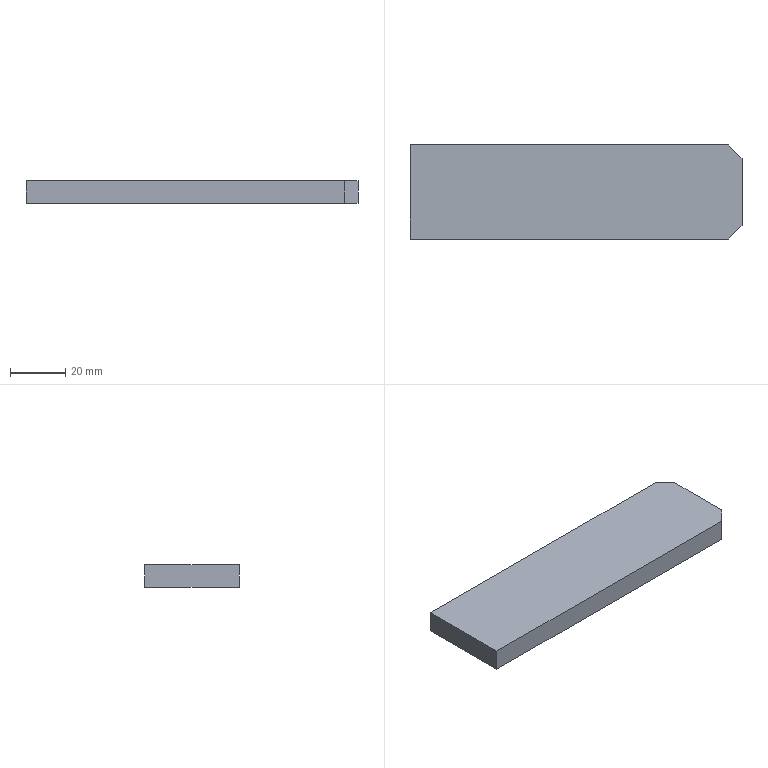Part | STEP file | ASND-0110-Body 1-1-1 | 1 solid | 8 faces | box 120 x 34 x 8 mm | volume 32440 mm3 | plane 8
STEP:
#1=CARTESIAN_POINT('',(0.,0.,0.));
#2=DIRECTION('',(0.,0.,1.));
#3=DIRECTION('',(1.,0.,0.));
#4=AXIS2_PLACEMENT_3D('',#1,#2,#3);
#5=CARTESIAN_POINT('',(115.,34.,8.));
#6=VERTEX_POINT('',#5);
#7=CARTESIAN_POINT('',(120.,29.,8.));
#8=VERTEX_POINT('',#7);
#9=CARTESIAN_POINT('',(115.,34.,8.));
#10=DIRECTION('',(0.7071,-0.7071,0.));
#11=VECTOR('',#10,1.);
#12=LINE('',#9,#11);
#13=CARTESIAN_POINT('',(117.5,31.5,0.));
#14=DIRECTION('',(0.7071,0.7071,0.));
#15=DIRECTION('',(-0.5774,0.5774,0.5774));
#16=AXIS2_PLACEMENT_3D('',#13,#14,#15);
#17=PLANE('',#16);
#18=CARTESIAN_POINT('',(7.506,4.491));
#19=DIRECTION('',(-0.8165,0.5774));
#20=VECTOR('',#19,1.);
#21=LINE('',#18,#20);
#22=(GEOMETRIC_REPRESENTATION_CONTEXT(2)PARAMETRIC_REPRESENTATION_CONTEXT()REPRESENTATION_CONTEXT('',''));
#23=DEFINITIONAL_REPRESENTATION('',(#21),#22);
#24=PCURVE('',#17,#23);
#25=CARTESIAN_POINT('',(50.,25.,8.));
#26=DIRECTION('',(0.,0.,1.));
#27=DIRECTION('',(0.7071,0.7071,0.));
#28=AXIS2_PLACEMENT_3D('',#25,#26,#27);
#29=PLANE('',#28);
#30=CARTESIAN_POINT('',(52.326,-39.598));
#31=DIRECTION('',(0.,-1.));
#32=VECTOR('',#31,1.);
#33=LINE('',#30,#32);
#34=(GEOMETRIC_REPRESENTATION_CONTEXT(2)PARAMETRIC_REPRESENTATION_CONTEXT()REPRESENTATION_CONTEXT('',''));
#35=DEFINITIONAL_REPRESENTATION('',(#33),#34);
#36=PCURVE('',#29,#35);
#37=SURFACE_CURVE('',#12,(#24,#36),.PCURVE_S1.);
#38=EDGE_CURVE('',#6,#8,#37,.T.);
#39=ORIENTED_EDGE('',*,*,#38,.T.);
#40=CARTESIAN_POINT('',(120.,29.,0.));
#41=VERTEX_POINT('',#40);
#42=CARTESIAN_POINT('',(120.,29.,8.));
#43=DIRECTION('',(0.,0.,-1.));
#44=VECTOR('',#43,1.);
#45=LINE('',#42,#44);
#46=CARTESIAN_POINT('',(1.732,8.573));
#47=DIRECTION('',(-0.5774,-0.8165));
#48=VECTOR('',#47,1.);
#49=LINE('',#46,#48);
#50=(GEOMETRIC_REPRESENTATION_CONTEXT(2)PARAMETRIC_REPRESENTATION_CONTEXT()REPRESENTATION_CONTEXT('',''));
#51=DEFINITIONAL_REPRESENTATION('',(#49),#50);
#52=PCURVE('',#17,#51);
#53=CARTESIAN_POINT('',(120.,50.,0.));
#54=DIRECTION('',(1.,0.,0.));
#55=DIRECTION('',(0.,0.7071,0.7071));
#56=AXIS2_PLACEMENT_3D('',#53,#54,#55);
#57=PLANE('',#56);
#58=CARTESIAN_POINT('',(-9.192,20.506));
#59=DIRECTION('',(-0.7071,-0.7071));
#60=VECTOR('',#59,1.);
#61=LINE('',#58,#60);
#62=(GEOMETRIC_REPRESENTATION_CONTEXT(2)PARAMETRIC_REPRESENTATION_CONTEXT()REPRESENTATION_CONTEXT('',''));
#63=DEFINITIONAL_REPRESENTATION('',(#61),#62);
#64=PCURVE('',#57,#63);
#65=SURFACE_CURVE('',#45,(#52,#64),.PCURVE_S1.);
#66=EDGE_CURVE('',#8,#41,#65,.T.);
#67=ORIENTED_EDGE('',*,*,#66,.T.);
#68=CARTESIAN_POINT('',(115.,34.,0.));
#69=VERTEX_POINT('',#68);
#70=CARTESIAN_POINT('',(120.,29.,0.));
#71=DIRECTION('',(-0.7071,0.7071,0.));
#72=VECTOR('',#71,1.);
#73=LINE('',#70,#72);
#74=CARTESIAN_POINT('',(-2.887,2.041));
#75=DIRECTION('',(0.8165,-0.5774));
#76=VECTOR('',#75,1.);
#77=LINE('',#74,#76);
#78=(GEOMETRIC_REPRESENTATION_CONTEXT(2)PARAMETRIC_REPRESENTATION_CONTEXT()REPRESENTATION_CONTEXT('',''));
#79=DEFINITIONAL_REPRESENTATION('',(#77),#78);
#80=PCURVE('',#17,#79);
#81=CARTESIAN_POINT('',(50.,25.,0.));
#82=DIRECTION('',(0.,0.,1.));
#83=DIRECTION('',(0.7071,0.7071,0.));
#84=AXIS2_PLACEMENT_3D('',#81,#82,#83);
#85=PLANE('',#84);
#86=CARTESIAN_POINT('',(52.326,-46.669));
#87=DIRECTION('',(0.,1.));
#88=VECTOR('',#87,1.);
#89=LINE('',#86,#88);
#90=(GEOMETRIC_REPRESENTATION_CONTEXT(2)PARAMETRIC_REPRESENTATION_CONTEXT()REPRESENTATION_CONTEXT('',''));
#91=DEFINITIONAL_REPRESENTATION('',(#89),#90);
#92=PCURVE('',#85,#91);
#93=SURFACE_CURVE('',#73,(#80,#92),.PCURVE_S1.);
#94=EDGE_CURVE('',#41,#69,#93,.T.);
#95=ORIENTED_EDGE('',*,*,#94,.T.);
#96=CARTESIAN_POINT('',(115.,34.,0.));
#97=DIRECTION('',(0.,0.,1.));
#98=VECTOR('',#97,1.);
#99=LINE('',#96,#98);
#100=CARTESIAN_POINT('',(2.887,-2.041));
#101=DIRECTION('',(0.5774,0.8165));
#102=VECTOR('',#101,1.);
#103=LINE('',#100,#102);
#104=(GEOMETRIC_REPRESENTATION_CONTEXT(2)PARAMETRIC_REPRESENTATION_CONTEXT()REPRESENTATION_CONTEXT('',''));
#105=DEFINITIONAL_REPRESENTATION('',(#103),#104);
#106=PCURVE('',#17,#105);
#107=CARTESIAN_POINT('',(0.,34.,0.));
#108=DIRECTION('',(0.,1.,0.));
#109=DIRECTION('',(0.7071,0.,0.7071));
#110=AXIS2_PLACEMENT_3D('',#107,#108,#109);
#111=PLANE('',#110);
#112=CARTESIAN_POINT('',(81.317,81.317));
#113=DIRECTION('',(0.7071,-0.7071));
#114=VECTOR('',#113,1.);
#115=LINE('',#112,#114);
#116=(GEOMETRIC_REPRESENTATION_CONTEXT(2)PARAMETRIC_REPRESENTATION_CONTEXT()REPRESENTATION_CONTEXT('',''));
#117=DEFINITIONAL_REPRESENTATION('',(#115),#116);
#118=PCURVE('',#111,#117);
#119=SURFACE_CURVE('',#99,(#106,#118),.PCURVE_S1.);
#120=EDGE_CURVE('',#69,#6,#119,.T.);
#121=ORIENTED_EDGE('',*,*,#120,.T.);
#122=EDGE_LOOP('',(#39,#67,#95,#121));
#123=FACE_BOUND('',#122,.T.);
#124=ADVANCED_FACE('',(#123),#17,.T.);
#125=ORIENTED_EDGE('',*,*,#120,.F.);
#126=CARTESIAN_POINT('',(0.,34.,0.));
#127=VERTEX_POINT('',#126);
#128=CARTESIAN_POINT('',(125.,34.,0.));
#129=DIRECTION('',(-1.,0.,0.));
#130=VECTOR('',#129,1.);
#131=LINE('',#128,#130);
#132=CARTESIAN_POINT('',(88.388,88.388));
#133=DIRECTION('',(-0.7071,-0.7071));
#134=VECTOR('',#133,1.);
#135=LINE('',#132,#134);
#136=(GEOMETRIC_REPRESENTATION_CONTEXT(2)PARAMETRIC_REPRESENTATION_CONTEXT()REPRESENTATION_CONTEXT('',''));
#137=DEFINITIONAL_REPRESENTATION('',(#135),#136);
#138=PCURVE('',#111,#137);
#139=CARTESIAN_POINT('',(59.397,-46.669));
#140=DIRECTION('',(-0.7071,0.7071));
#141=VECTOR('',#140,1.);
#142=LINE('',#139,#141);
#143=(GEOMETRIC_REPRESENTATION_CONTEXT(2)PARAMETRIC_REPRESENTATION_CONTEXT()REPRESENTATION_CONTEXT('',''));
#144=DEFINITIONAL_REPRESENTATION('',(#142),#143);
#145=PCURVE('',#85,#144);
#146=SURFACE_CURVE('',#131,(#138,#145),.PCURVE_S1.);
#147=EDGE_CURVE('',#69,#127,#146,.T.);
#148=ORIENTED_EDGE('',*,*,#147,.T.);
#149=CARTESIAN_POINT('',(0.,34.,8.));
#150=VERTEX_POINT('',#149);
#151=CARTESIAN_POINT('',(0.,34.,0.));
#152=DIRECTION('',(0.,0.,1.));
#153=VECTOR('',#152,1.);
#154=LINE('',#151,#153);
#155=CARTESIAN_POINT('',(0.,0.));
#156=DIRECTION('',(0.7071,-0.7071));
#157=VECTOR('',#156,1.);
#158=LINE('',#155,#157);
#159=(GEOMETRIC_REPRESENTATION_CONTEXT(2)PARAMETRIC_REPRESENTATION_CONTEXT()REPRESENTATION_CONTEXT('',''));
#160=DEFINITIONAL_REPRESENTATION('',(#158),#159);
#161=PCURVE('',#111,#160);
#162=CARTESIAN_POINT('',(0.,0.,0.));
#163=DIRECTION('',(-1.,0.,0.));
#164=DIRECTION('',(0.,0.7071,0.7071));
#165=AXIS2_PLACEMENT_3D('',#162,#163,#164);
#166=PLANE('',#165);
#167=CARTESIAN_POINT('',(24.042,24.042));
#168=DIRECTION('',(0.7071,-0.7071));
#169=VECTOR('',#168,1.);
#170=LINE('',#167,#169);
#171=(GEOMETRIC_REPRESENTATION_CONTEXT(2)PARAMETRIC_REPRESENTATION_CONTEXT()REPRESENTATION_CONTEXT('',''));
#172=DEFINITIONAL_REPRESENTATION('',(#170),#171);
#173=PCURVE('',#166,#172);
#174=SURFACE_CURVE('',#154,(#161,#173),.PCURVE_S1.);
#175=EDGE_CURVE('',#127,#150,#174,.T.);
#176=ORIENTED_EDGE('',*,*,#175,.T.);
#177=CARTESIAN_POINT('',(0.,34.,8.));
#178=DIRECTION('',(1.,0.,0.));
#179=VECTOR('',#178,1.);
#180=LINE('',#177,#179);
#181=CARTESIAN_POINT('',(5.657,-5.657));
#182=DIRECTION('',(0.7071,0.7071));
#183=VECTOR('',#182,1.);
#184=LINE('',#181,#183);
#185=(GEOMETRIC_REPRESENTATION_CONTEXT(2)PARAMETRIC_REPRESENTATION_CONTEXT()REPRESENTATION_CONTEXT('',''));
#186=DEFINITIONAL_REPRESENTATION('',(#184),#185);
#187=PCURVE('',#111,#186);
#188=CARTESIAN_POINT('',(-28.991,41.719));
#189=DIRECTION('',(0.7071,-0.7071));
#190=VECTOR('',#189,1.);
#191=LINE('',#188,#190);
#192=(GEOMETRIC_REPRESENTATION_CONTEXT(2)PARAMETRIC_REPRESENTATION_CONTEXT()REPRESENTATION_CONTEXT('',''));
#193=DEFINITIONAL_REPRESENTATION('',(#191),#192);
#194=PCURVE('',#29,#193);
#195=SURFACE_CURVE('',#180,(#187,#194),.PCURVE_S1.);
#196=EDGE_CURVE('',#150,#6,#195,.T.);
#197=ORIENTED_EDGE('',*,*,#196,.T.);
#198=EDGE_LOOP('',(#125,#148,#176,#197));
#199=FACE_BOUND('',#198,.T.);
#200=ADVANCED_FACE('',(#199),#111,.T.);
#201=ORIENTED_EDGE('',*,*,#94,.F.);
#202=CARTESIAN_POINT('',(120.,5.,0.));
#203=VERTEX_POINT('',#202);
#204=CARTESIAN_POINT('',(120.,5.,0.));
#205=DIRECTION('',(0.,1.,0.));
#206=VECTOR('',#205,1.);
#207=LINE('',#204,#206);
#208=CARTESIAN_POINT('',(35.355,-63.64));
#209=DIRECTION('',(0.7071,0.7071));
#210=VECTOR('',#209,1.);
#211=LINE('',#208,#210);
#212=(GEOMETRIC_REPRESENTATION_CONTEXT(2)PARAMETRIC_REPRESENTATION_CONTEXT()REPRESENTATION_CONTEXT('',''));
#213=DEFINITIONAL_REPRESENTATION('',(#211),#212);
#214=PCURVE('',#85,#213);
#215=CARTESIAN_POINT('',(-31.82,31.82));
#216=DIRECTION('',(0.7071,-0.7071));
#217=VECTOR('',#216,1.);
#218=LINE('',#215,#217);
#219=(GEOMETRIC_REPRESENTATION_CONTEXT(2)PARAMETRIC_REPRESENTATION_CONTEXT()REPRESENTATION_CONTEXT('',''));
#220=DEFINITIONAL_REPRESENTATION('',(#218),#219);
#221=PCURVE('',#57,#220);
#222=SURFACE_CURVE('',#207,(#214,#221),.PCURVE_S1.);
#223=EDGE_CURVE('',#203,#41,#222,.T.);
#224=ORIENTED_EDGE('',*,*,#223,.F.);
#225=CARTESIAN_POINT('',(115.,0.,0.));
#226=VERTEX_POINT('',#225);
#227=CARTESIAN_POINT('',(115.,0.,0.));
#228=DIRECTION('',(0.7071,0.7071,0.));
#229=VECTOR('',#228,1.);
#230=LINE('',#227,#229);
#231=CARTESIAN_POINT('',(28.284,-63.64));
#232=DIRECTION('',(1.,0.));
#233=VECTOR('',#232,1.);
#234=LINE('',#231,#233);
#235=(GEOMETRIC_REPRESENTATION_CONTEXT(2)PARAMETRIC_REPRESENTATION_CONTEXT()REPRESENTATION_CONTEXT('',''));
#236=DEFINITIONAL_REPRESENTATION('',(#234),#235);
#237=PCURVE('',#85,#236);
#238=CARTESIAN_POINT('',(117.5,2.5,0.));
#239=DIRECTION('',(0.7071,-0.7071,0.));
#240=DIRECTION('',(0.5774,0.5774,0.5774));
#241=AXIS2_PLACEMENT_3D('',#238,#239,#240);
#242=PLANE('',#241);
#243=CARTESIAN_POINT('',(-2.887,2.041));
#244=DIRECTION('',(0.8165,-0.5774));
#245=VECTOR('',#244,1.);
#246=LINE('',#243,#245);
#247=(GEOMETRIC_REPRESENTATION_CONTEXT(2)PARAMETRIC_REPRESENTATION_CONTEXT()REPRESENTATION_CONTEXT('',''));
#248=DEFINITIONAL_REPRESENTATION('',(#246),#247);
#249=PCURVE('',#242,#248);
#250=SURFACE_CURVE('',#230,(#237,#249),.PCURVE_S1.);
#251=EDGE_CURVE('',#226,#203,#250,.T.);
#252=ORIENTED_EDGE('',*,*,#251,.F.);
#253=CARTESIAN_POINT('',(0.,0.,0.));
#254=VERTEX_POINT('',#253);
#255=CARTESIAN_POINT('',(0.,0.,0.));
#256=DIRECTION('',(1.,0.,0.));
#257=VECTOR('',#256,1.);
#258=LINE('',#255,#257);
#259=CARTESIAN_POINT('',(-53.033,17.678));
#260=DIRECTION('',(0.7071,-0.7071));
#261=VECTOR('',#260,1.);
#262=LINE('',#259,#261);
#263=(GEOMETRIC_REPRESENTATION_CONTEXT(2)PARAMETRIC_REPRESENTATION_CONTEXT()REPRESENTATION_CONTEXT('',''));
#264=DEFINITIONAL_REPRESENTATION('',(#262),#263);
#265=PCURVE('',#85,#264);
#266=CARTESIAN_POINT('',(100.,0.,0.));
#267=DIRECTION('',(0.,-1.,0.));
#268=DIRECTION('',(0.7071,0.,0.7071));
#269=AXIS2_PLACEMENT_3D('',#266,#267,#268);
#270=PLANE('',#269);
#271=CARTESIAN_POINT('',(-70.711,70.711));
#272=DIRECTION('',(0.7071,-0.7071));
#273=VECTOR('',#272,1.);
#274=LINE('',#271,#273);
#275=(GEOMETRIC_REPRESENTATION_CONTEXT(2)PARAMETRIC_REPRESENTATION_CONTEXT()REPRESENTATION_CONTEXT('',''));
#276=DEFINITIONAL_REPRESENTATION('',(#274),#275);
#277=PCURVE('',#270,#276);
#278=SURFACE_CURVE('',#258,(#265,#277),.PCURVE_S1.);
#279=EDGE_CURVE('',#254,#226,#278,.T.);
#280=ORIENTED_EDGE('',*,*,#279,.F.);
#281=CARTESIAN_POINT('',(0.,50.,0.));
#282=DIRECTION('',(0.,-1.,0.));
#283=VECTOR('',#282,1.);
#284=LINE('',#281,#283);
#285=CARTESIAN_POINT('',(-17.678,53.033));
#286=DIRECTION('',(-0.7071,-0.7071));
#287=VECTOR('',#286,1.);
#288=LINE('',#285,#287);
#289=(GEOMETRIC_REPRESENTATION_CONTEXT(2)PARAMETRIC_REPRESENTATION_CONTEXT()REPRESENTATION_CONTEXT('',''));
#290=DEFINITIONAL_REPRESENTATION('',(#288),#289);
#291=PCURVE('',#85,#290);
#292=CARTESIAN_POINT('',(35.355,35.355));
#293=DIRECTION('',(-0.7071,-0.7071));
#294=VECTOR('',#293,1.);
#295=LINE('',#292,#294);
#296=(GEOMETRIC_REPRESENTATION_CONTEXT(2)PARAMETRIC_REPRESENTATION_CONTEXT()REPRESENTATION_CONTEXT('',''));
#297=DEFINITIONAL_REPRESENTATION('',(#295),#296);
#298=PCURVE('',#166,#297);
#299=SURFACE_CURVE('',#284,(#291,#298),.PCURVE_S1.);
#300=EDGE_CURVE('',#127,#254,#299,.T.);
#301=ORIENTED_EDGE('',*,*,#300,.F.);
#302=ORIENTED_EDGE('',*,*,#147,.F.);
#303=EDGE_LOOP('',(#201,#224,#252,#280,#301,#302));
#304=FACE_BOUND('',#303,.T.);
#305=ADVANCED_FACE('',(#304),#85,.F.);
#306=CARTESIAN_POINT('',(120.,5.,8.));
#307=VERTEX_POINT('',#306);
#308=CARTESIAN_POINT('',(115.,0.,8.));
#309=VERTEX_POINT('',#308);
#310=CARTESIAN_POINT('',(120.,5.,8.));
#311=DIRECTION('',(-0.7071,-0.7071,0.));
#312=VECTOR('',#311,1.);
#313=LINE('',#310,#312);
#314=CARTESIAN_POINT('',(7.506,4.491));
#315=DIRECTION('',(-0.8165,0.5774));
#316=VECTOR('',#315,1.);
#317=LINE('',#314,#316);
#318=(GEOMETRIC_REPRESENTATION_CONTEXT(2)PARAMETRIC_REPRESENTATION_CONTEXT()REPRESENTATION_CONTEXT('',''));
#319=DEFINITIONAL_REPRESENTATION('',(#317),#318);
#320=PCURVE('',#242,#319);
#321=CARTESIAN_POINT('',(35.355,-63.64));
#322=DIRECTION('',(-1.,0.));
#323=VECTOR('',#322,1.);
#324=LINE('',#321,#323);
#325=(GEOMETRIC_REPRESENTATION_CONTEXT(2)PARAMETRIC_REPRESENTATION_CONTEXT()REPRESENTATION_CONTEXT('',''));
#326=DEFINITIONAL_REPRESENTATION('',(#324),#325);
#327=PCURVE('',#29,#326);
#328=SURFACE_CURVE('',#313,(#320,#327),.PCURVE_S1.);
#329=EDGE_CURVE('',#307,#309,#328,.T.);
#330=ORIENTED_EDGE('',*,*,#329,.T.);
#331=CARTESIAN_POINT('',(115.,0.,8.));
#332=DIRECTION('',(0.,0.,-1.));
#333=VECTOR('',#332,1.);
#334=LINE('',#331,#333);
#335=CARTESIAN_POINT('',(1.732,8.573));
#336=DIRECTION('',(-0.5774,-0.8165));
#337=VECTOR('',#336,1.);
#338=LINE('',#335,#337);
#339=(GEOMETRIC_REPRESENTATION_CONTEXT(2)PARAMETRIC_REPRESENTATION_CONTEXT()REPRESENTATION_CONTEXT('',''));
#340=DEFINITIONAL_REPRESENTATION('',(#338),#339);
#341=PCURVE('',#242,#340);
#342=CARTESIAN_POINT('',(16.263,-4.95));
#343=DIRECTION('',(-0.7071,-0.7071));
#344=VECTOR('',#343,1.);
#345=LINE('',#342,#344);
#346=(GEOMETRIC_REPRESENTATION_CONTEXT(2)PARAMETRIC_REPRESENTATION_CONTEXT()REPRESENTATION_CONTEXT('',''));
#347=DEFINITIONAL_REPRESENTATION('',(#345),#346);
#348=PCURVE('',#270,#347);
#349=SURFACE_CURVE('',#334,(#341,#348),.PCURVE_S1.);
#350=EDGE_CURVE('',#309,#226,#349,.T.);
#351=ORIENTED_EDGE('',*,*,#350,.T.);
#352=ORIENTED_EDGE('',*,*,#251,.T.);
#353=CARTESIAN_POINT('',(120.,5.,0.));
#354=DIRECTION('',(0.,0.,1.));
#355=VECTOR('',#354,1.);
#356=LINE('',#353,#355);
#357=CARTESIAN_POINT('',(2.887,-2.041));
#358=DIRECTION('',(0.5774,0.8165));
#359=VECTOR('',#358,1.);
#360=LINE('',#357,#359);
#361=(GEOMETRIC_REPRESENTATION_CONTEXT(2)PARAMETRIC_REPRESENTATION_CONTEXT()REPRESENTATION_CONTEXT('',''));
#362=DEFINITIONAL_REPRESENTATION('',(#360),#361);
#363=PCURVE('',#242,#362);
#364=CARTESIAN_POINT('',(-31.82,31.82));
#365=DIRECTION('',(0.7071,0.7071));
#366=VECTOR('',#365,1.);
#367=LINE('',#364,#366);
#368=(GEOMETRIC_REPRESENTATION_CONTEXT(2)PARAMETRIC_REPRESENTATION_CONTEXT()REPRESENTATION_CONTEXT('',''));
#369=DEFINITIONAL_REPRESENTATION('',(#367),#368);
#370=PCURVE('',#57,#369);
#371=SURFACE_CURVE('',#356,(#363,#370),.PCURVE_S1.);
#372=EDGE_CURVE('',#203,#307,#371,.T.);
#373=ORIENTED_EDGE('',*,*,#372,.T.);
#374=EDGE_LOOP('',(#330,#351,#352,#373));
#375=FACE_BOUND('',#374,.T.);
#376=ADVANCED_FACE('',(#375),#242,.T.);
#377=ORIENTED_EDGE('',*,*,#350,.F.);
#378=CARTESIAN_POINT('',(0.,0.,8.));
#379=VERTEX_POINT('',#378);
#380=CARTESIAN_POINT('',(125.,0.,8.));
#381=DIRECTION('',(-1.,0.,0.));
#382=VECTOR('',#381,1.);
#383=LINE('',#380,#382);
#384=CARTESIAN_POINT('',(23.335,-12.021));
#385=DIRECTION('',(-0.7071,0.7071));
#386=VECTOR('',#385,1.);
#387=LINE('',#384,#386);
#388=(GEOMETRIC_REPRESENTATION_CONTEXT(2)PARAMETRIC_REPRESENTATION_CONTEXT()REPRESENTATION_CONTEXT('',''));
#389=DEFINITIONAL_REPRESENTATION('',(#387),#388);
#390=PCURVE('',#270,#389);
#391=CARTESIAN_POINT('',(35.355,-70.711));
#392=DIRECTION('',(-0.7071,0.7071));
#393=VECTOR('',#392,1.);
#394=LINE('',#391,#393);
#395=(GEOMETRIC_REPRESENTATION_CONTEXT(2)PARAMETRIC_REPRESENTATION_CONTEXT()REPRESENTATION_CONTEXT('',''));
#396=DEFINITIONAL_REPRESENTATION('',(#394),#395);
#397=PCURVE('',#29,#396);
#398=SURFACE_CURVE('',#383,(#390,#397),.PCURVE_S1.);
#399=EDGE_CURVE('',#309,#379,#398,.T.);
#400=ORIENTED_EDGE('',*,*,#399,.T.);
#401=CARTESIAN_POINT('',(0.,0.,0.));
#402=DIRECTION('',(0.,0.,1.));
#403=VECTOR('',#402,1.);
#404=LINE('',#401,#403);
#405=CARTESIAN_POINT('',(-70.711,70.711));
#406=DIRECTION('',(0.7071,0.7071));
#407=VECTOR('',#406,1.);
#408=LINE('',#405,#407);
#409=(GEOMETRIC_REPRESENTATION_CONTEXT(2)PARAMETRIC_REPRESENTATION_CONTEXT()REPRESENTATION_CONTEXT('',''));
#410=DEFINITIONAL_REPRESENTATION('',(#408),#409);
#411=PCURVE('',#270,#410);
#412=CARTESIAN_POINT('',(0.,0.));
#413=DIRECTION('',(0.7071,-0.7071));
#414=VECTOR('',#413,1.);
#415=LINE('',#412,#414);
#416=(GEOMETRIC_REPRESENTATION_CONTEXT(2)PARAMETRIC_REPRESENTATION_CONTEXT()REPRESENTATION_CONTEXT('',''));
#417=DEFINITIONAL_REPRESENTATION('',(#415),#416);
#418=PCURVE('',#166,#417);
#419=SURFACE_CURVE('',#404,(#411,#418),.PCURVE_S1.);
#420=EDGE_CURVE('',#254,#379,#419,.T.);
#421=ORIENTED_EDGE('',*,*,#420,.F.);
#422=ORIENTED_EDGE('',*,*,#279,.T.);
#423=EDGE_LOOP('',(#377,#400,#421,#422));
#424=FACE_BOUND('',#423,.T.);
#425=ADVANCED_FACE('',(#424),#270,.T.);
#426=CARTESIAN_POINT('',(0.,0.,8.));
#427=DIRECTION('',(0.,1.,0.));
#428=VECTOR('',#427,1.);
#429=LINE('',#426,#428);
#430=CARTESIAN_POINT('',(5.657,-5.657));
#431=DIRECTION('',(0.7071,0.7071));
#432=VECTOR('',#431,1.);
#433=LINE('',#430,#432);
#434=(GEOMETRIC_REPRESENTATION_CONTEXT(2)PARAMETRIC_REPRESENTATION_CONTEXT()REPRESENTATION_CONTEXT('',''));
#435=DEFINITIONAL_REPRESENTATION('',(#433),#434);
#436=PCURVE('',#166,#435);
#437=CARTESIAN_POINT('',(-53.033,17.678));
#438=DIRECTION('',(0.7071,0.7071));
#439=VECTOR('',#438,1.);
#440=LINE('',#437,#439);
#441=(GEOMETRIC_REPRESENTATION_CONTEXT(2)PARAMETRIC_REPRESENTATION_CONTEXT()REPRESENTATION_CONTEXT('',''));
#442=DEFINITIONAL_REPRESENTATION('',(#440),#441);
#443=PCURVE('',#29,#442);
#444=SURFACE_CURVE('',#429,(#436,#443),.PCURVE_S1.);
#445=EDGE_CURVE('',#379,#150,#444,.T.);
#446=ORIENTED_EDGE('',*,*,#445,.T.);
#447=ORIENTED_EDGE('',*,*,#175,.F.);
#448=ORIENTED_EDGE('',*,*,#300,.T.);
#449=ORIENTED_EDGE('',*,*,#420,.T.);
#450=EDGE_LOOP('',(#446,#447,#448,#449));
#451=FACE_BOUND('',#450,.T.);
#452=ADVANCED_FACE('',(#451),#166,.T.);
#453=ORIENTED_EDGE('',*,*,#66,.F.);
#454=CARTESIAN_POINT('',(120.,45.,8.));
#455=DIRECTION('',(0.,-1.,0.));
#456=VECTOR('',#455,1.);
#457=LINE('',#454,#456);
#458=CARTESIAN_POINT('',(2.121,9.192));
#459=DIRECTION('',(-0.7071,0.7071));
#460=VECTOR('',#459,1.);
#461=LINE('',#458,#460);
#462=(GEOMETRIC_REPRESENTATION_CONTEXT(2)PARAMETRIC_REPRESENTATION_CONTEXT()REPRESENTATION_CONTEXT('',''));
#463=DEFINITIONAL_REPRESENTATION('',(#461),#462);
#464=PCURVE('',#57,#463);
#465=CARTESIAN_POINT('',(63.64,-35.355));
#466=DIRECTION('',(-0.7071,-0.7071));
#467=VECTOR('',#466,1.);
#468=LINE('',#465,#467);
#469=(GEOMETRIC_REPRESENTATION_CONTEXT(2)PARAMETRIC_REPRESENTATION_CONTEXT()REPRESENTATION_CONTEXT('',''));
#470=DEFINITIONAL_REPRESENTATION('',(#468),#469);
#471=PCURVE('',#29,#470);
#472=SURFACE_CURVE('',#457,(#464,#471),.PCURVE_S1.);
#473=EDGE_CURVE('',#8,#307,#472,.T.);
#474=ORIENTED_EDGE('',*,*,#473,.T.);
#475=ORIENTED_EDGE('',*,*,#372,.F.);
#476=ORIENTED_EDGE('',*,*,#223,.T.);
#477=EDGE_LOOP('',(#453,#474,#475,#476));
#478=FACE_BOUND('',#477,.T.);
#479=ADVANCED_FACE('',(#478),#57,.T.);
#480=ORIENTED_EDGE('',*,*,#38,.F.);
#481=ORIENTED_EDGE('',*,*,#196,.F.);
#482=ORIENTED_EDGE('',*,*,#445,.F.);
#483=ORIENTED_EDGE('',*,*,#399,.F.);
#484=ORIENTED_EDGE('',*,*,#329,.F.);
#485=ORIENTED_EDGE('',*,*,#473,.F.);
#486=EDGE_LOOP('',(#480,#481,#482,#483,#484,#485));
#487=FACE_BOUND('',#486,.T.);
#488=ADVANCED_FACE('',(#487),#29,.T.);
#489=CLOSED_SHELL('',(#124,#200,#305,#376,#425,#452,#479,#488));
#490=MANIFOLD_SOLID_BREP('',#489);
#491=(LENGTH_UNIT()NAMED_UNIT(*)SI_UNIT(.MILLI.,.METRE.));
#492=UNCERTAINTY_MEASURE_WITH_UNIT(LENGTH_MEASURE(0.0000001),#491,'','');
#493=(NAMED_UNIT(*)PLANE_ANGLE_UNIT()SI_UNIT($,.RADIAN.));
#494=(NAMED_UNIT(*)SI_UNIT($,.STERADIAN.)SOLID_ANGLE_UNIT());
#495=(GEOMETRIC_REPRESENTATION_CONTEXT(3)GLOBAL_UNCERTAINTY_ASSIGNED_CONTEXT((#492))GLOBAL_UNIT_ASSIGNED_CONTEXT((#491,#493,#494))REPRESENTATION_CONTEXT('',''));
#496=ADVANCED_BREP_SHAPE_REPRESENTATION('',(#4,#490),#495);